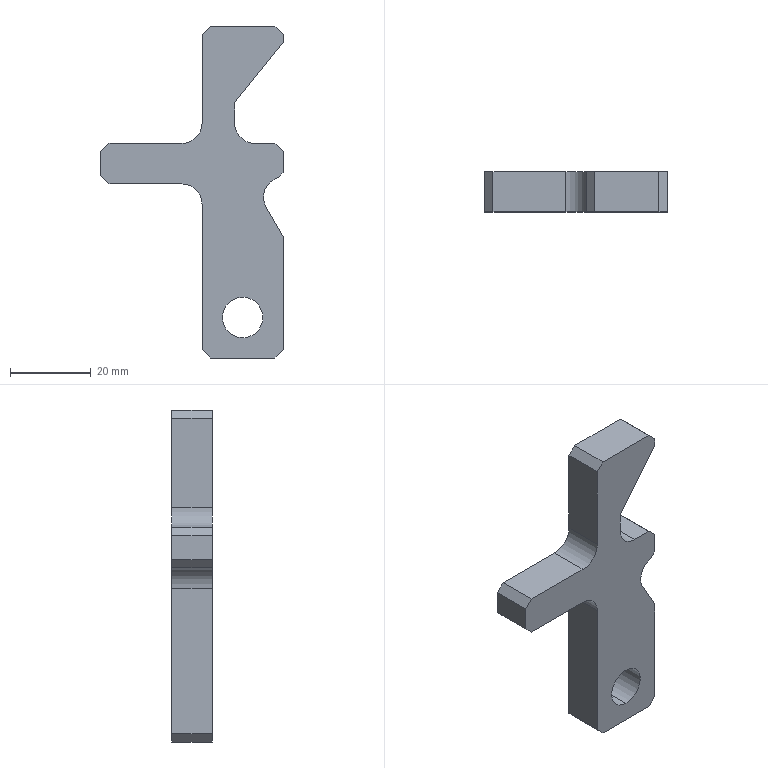Part | STEP file | 0217_204_Block | 1 solid | 30 faces | box 45 x 9.9 x 82 mm | volume 15419 mm3 | plane 24 | cylinder 6 | commonest cylinder face diameters 10 x6